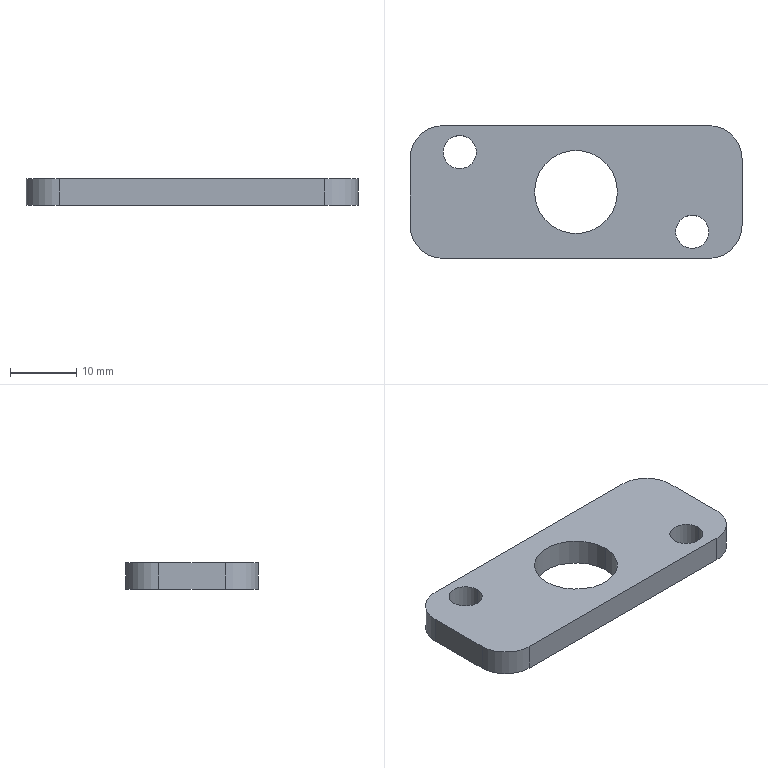Part | SolidWorks | features Extrusion 1 | 1 solid | 16 faces | box 50 x 20 x 4 mm | volume 3266 mm3 | cylinder 10 | plane 6 | commonest cylinder face diameters 5 x4 10 x4 12.5 x2
STEP:
#1=CARTESIAN_POINT('',(-6.25,0.,-2.));
#2=VERTEX_POINT('',#1);
#3=CARTESIAN_POINT('',(6.25,0.,-2.));
#4=VERTEX_POINT('',#3);
#5=CARTESIAN_POINT('',(0.,0.,-2.));
#6=DIRECTION('',(0.,0.,1.));
#7=DIRECTION('',(-1.,0.,0.));
#8=AXIS2_PLACEMENT_3D('',#5,#6,#7);
#9=CIRCLE('',#8,6.25);
#10=EDGE_CURVE('',#2,#4,#9,.T.);
#11=ORIENTED_EDGE('',*,*,#10,.F.);
#12=CARTESIAN_POINT('',(-6.25,0.,2.));
#13=VERTEX_POINT('',#12);
#14=CARTESIAN_POINT('',(-6.25,0.,-2.));
#15=DIRECTION('',(0.,0.,1.));
#16=VECTOR('',#15,1000.);
#17=LINE('',#14,#16);
#18=EDGE_CURVE('',#2,#13,#17,.T.);
#19=ORIENTED_EDGE('',*,*,#18,.T.);
#20=CARTESIAN_POINT('',(6.25,0.,2.));
#21=VERTEX_POINT('',#20);
#22=CARTESIAN_POINT('',(0.,0.,2.));
#23=DIRECTION('',(0.,0.,1.));
#24=DIRECTION('',(-1.,0.,0.));
#25=AXIS2_PLACEMENT_3D('',#22,#23,#24);
#26=CIRCLE('',#25,6.25);
#27=EDGE_CURVE('',#13,#21,#26,.T.);
#28=ORIENTED_EDGE('',*,*,#27,.T.);
#29=CARTESIAN_POINT('',(6.25,0.,-2.));
#30=DIRECTION('',(0.,0.,1.));
#31=VECTOR('',#30,1000.);
#32=LINE('',#29,#31);
#33=EDGE_CURVE('',#4,#21,#32,.T.);
#34=ORIENTED_EDGE('',*,*,#33,.F.);
#35=EDGE_LOOP('',(#11,#19,#28,#34));
#36=FACE_OUTER_BOUND('',#35,.T.);
#37=CARTESIAN_POINT('',(0.,0.,-2.));
#38=DIRECTION('',(0.,0.,1.));
#39=DIRECTION('',(1.,0.,0.));
#40=AXIS2_PLACEMENT_3D('',#37,#38,#39);
#41=CYLINDRICAL_SURFACE('',#40,6.25);
#42=ADVANCED_FACE('',(#36),#41,.F.);
#43=CARTESIAN_POINT('',(15.,-6.,-2.));
#44=VERTEX_POINT('',#43);
#45=CARTESIAN_POINT('',(20.,-6.,-2.));
#46=VERTEX_POINT('',#45);
#47=CARTESIAN_POINT('',(17.5,-6.,-2.));
#48=DIRECTION('',(0.,0.,1.));
#49=DIRECTION('',(-1.,0.,0.));
#50=AXIS2_PLACEMENT_3D('',#47,#48,#49);
#51=CIRCLE('',#50,2.5);
#52=EDGE_CURVE('',#44,#46,#51,.T.);
#53=ORIENTED_EDGE('',*,*,#52,.F.);
#54=CARTESIAN_POINT('',(15.,-6.,2.));
#55=VERTEX_POINT('',#54);
#56=CARTESIAN_POINT('',(15.,-6.,-2.));
#57=DIRECTION('',(0.,0.,1.));
#58=VECTOR('',#57,1000.);
#59=LINE('',#56,#58);
#60=EDGE_CURVE('',#44,#55,#59,.T.);
#61=ORIENTED_EDGE('',*,*,#60,.T.);
#62=CARTESIAN_POINT('',(20.,-6.,2.));
#63=VERTEX_POINT('',#62);
#64=CARTESIAN_POINT('',(17.5,-6.,2.));
#65=DIRECTION('',(0.,0.,1.));
#66=DIRECTION('',(-1.,0.,0.));
#67=AXIS2_PLACEMENT_3D('',#64,#65,#66);
#68=CIRCLE('',#67,2.5);
#69=EDGE_CURVE('',#55,#63,#68,.T.);
#70=ORIENTED_EDGE('',*,*,#69,.T.);
#71=CARTESIAN_POINT('',(20.,-6.,-2.));
#72=DIRECTION('',(0.,0.,1.));
#73=VECTOR('',#72,1000.);
#74=LINE('',#71,#73);
#75=EDGE_CURVE('',#46,#63,#74,.T.);
#76=ORIENTED_EDGE('',*,*,#75,.F.);
#77=EDGE_LOOP('',(#53,#61,#70,#76));
#78=FACE_OUTER_BOUND('',#77,.T.);
#79=CARTESIAN_POINT('',(17.5,-6.,-2.));
#80=DIRECTION('',(0.,0.,1.));
#81=DIRECTION('',(1.,0.,0.));
#82=AXIS2_PLACEMENT_3D('',#79,#80,#81);
#83=CYLINDRICAL_SURFACE('',#82,2.5);
#84=ADVANCED_FACE('',(#78),#83,.F.);
#85=CARTESIAN_POINT('',(-20.,6.,-2.));
#86=VERTEX_POINT('',#85);
#87=CARTESIAN_POINT('',(-15.,6.,-2.));
#88=VERTEX_POINT('',#87);
#89=CARTESIAN_POINT('',(-17.5,6.,-2.));
#90=DIRECTION('',(0.,0.,1.));
#91=DIRECTION('',(-1.,0.,0.));
#92=AXIS2_PLACEMENT_3D('',#89,#90,#91);
#93=CIRCLE('',#92,2.5);
#94=EDGE_CURVE('',#86,#88,#93,.T.);
#95=ORIENTED_EDGE('',*,*,#94,.F.);
#96=CARTESIAN_POINT('',(-20.,6.,2.));
#97=VERTEX_POINT('',#96);
#98=CARTESIAN_POINT('',(-20.,6.,-2.));
#99=DIRECTION('',(0.,0.,1.));
#100=VECTOR('',#99,1000.);
#101=LINE('',#98,#100);
#102=EDGE_CURVE('',#86,#97,#101,.T.);
#103=ORIENTED_EDGE('',*,*,#102,.T.);
#104=CARTESIAN_POINT('',(-15.,6.,2.));
#105=VERTEX_POINT('',#104);
#106=CARTESIAN_POINT('',(-17.5,6.,2.));
#107=DIRECTION('',(0.,0.,1.));
#108=DIRECTION('',(-1.,0.,0.));
#109=AXIS2_PLACEMENT_3D('',#106,#107,#108);
#110=CIRCLE('',#109,2.5);
#111=EDGE_CURVE('',#97,#105,#110,.T.);
#112=ORIENTED_EDGE('',*,*,#111,.T.);
#113=CARTESIAN_POINT('',(-15.,6.,-2.));
#114=DIRECTION('',(0.,0.,1.));
#115=VECTOR('',#114,1000.);
#116=LINE('',#113,#115);
#117=EDGE_CURVE('',#88,#105,#116,.T.);
#118=ORIENTED_EDGE('',*,*,#117,.F.);
#119=EDGE_LOOP('',(#95,#103,#112,#118));
#120=FACE_OUTER_BOUND('',#119,.T.);
#121=CARTESIAN_POINT('',(-17.5,6.,-2.));
#122=DIRECTION('',(0.,0.,1.));
#123=DIRECTION('',(1.,0.,0.));
#124=AXIS2_PLACEMENT_3D('',#121,#122,#123);
#125=CYLINDRICAL_SURFACE('',#124,2.5);
#126=ADVANCED_FACE('',(#120),#125,.F.);
#127=CARTESIAN_POINT('',(-25.,-5.,2.));
#128=VERTEX_POINT('',#127);
#129=CARTESIAN_POINT('',(-20.,-10.,2.));
#130=VERTEX_POINT('',#129);
#131=CARTESIAN_POINT('',(-20.,-5.,2.));
#132=DIRECTION('',(0.,0.,1.));
#133=DIRECTION('',(1.,0.,0.));
#134=AXIS2_PLACEMENT_3D('',#131,#132,#133);
#135=CIRCLE('',#134,5.);
#136=EDGE_CURVE('',#128,#130,#135,.T.);
#137=ORIENTED_EDGE('',*,*,#136,.F.);
#138=CARTESIAN_POINT('',(-25.,-5.,-2.));
#139=VERTEX_POINT('',#138);
#140=CARTESIAN_POINT('',(-25.,-5.,-2.));
#141=DIRECTION('',(0.,0.,1.));
#142=VECTOR('',#141,1000.);
#143=LINE('',#140,#142);
#144=EDGE_CURVE('',#139,#128,#143,.T.);
#145=ORIENTED_EDGE('',*,*,#144,.F.);
#146=CARTESIAN_POINT('',(-20.,-10.,-2.));
#147=VERTEX_POINT('',#146);
#148=CARTESIAN_POINT('',(-20.,-5.,-2.));
#149=DIRECTION('',(0.,0.,1.));
#150=DIRECTION('',(1.,0.,0.));
#151=AXIS2_PLACEMENT_3D('',#148,#149,#150);
#152=CIRCLE('',#151,5.);
#153=EDGE_CURVE('',#139,#147,#152,.T.);
#154=ORIENTED_EDGE('',*,*,#153,.T.);
#155=CARTESIAN_POINT('',(-20.,-10.,-2.));
#156=DIRECTION('',(0.,0.,1.));
#157=VECTOR('',#156,1000.);
#158=LINE('',#155,#157);
#159=EDGE_CURVE('',#147,#130,#158,.T.);
#160=ORIENTED_EDGE('',*,*,#159,.T.);
#161=EDGE_LOOP('',(#137,#145,#154,#160));
#162=FACE_OUTER_BOUND('',#161,.T.);
#163=CARTESIAN_POINT('',(-20.,-5.,-2.));
#164=DIRECTION('',(0.,0.,1.));
#165=DIRECTION('',(1.,0.,0.));
#166=AXIS2_PLACEMENT_3D('',#163,#164,#165);
#167=CYLINDRICAL_SURFACE('',#166,5.);
#168=ADVANCED_FACE('',(#162),#167,.T.);
#169=CARTESIAN_POINT('',(-25.,5.,2.));
#170=VERTEX_POINT('',#169);
#171=CARTESIAN_POINT('',(-25.,5.,2.));
#172=DIRECTION('',(0.,-1.,0.));
#173=VECTOR('',#172,1000.);
#174=LINE('',#171,#173);
#175=EDGE_CURVE('',#170,#128,#174,.T.);
#176=ORIENTED_EDGE('',*,*,#175,.F.);
#177=CARTESIAN_POINT('',(-25.,5.,-2.));
#178=VERTEX_POINT('',#177);
#179=CARTESIAN_POINT('',(-25.,5.,-2.));
#180=DIRECTION('',(0.,0.,1.));
#181=VECTOR('',#180,1000.);
#182=LINE('',#179,#181);
#183=EDGE_CURVE('',#178,#170,#182,.T.);
#184=ORIENTED_EDGE('',*,*,#183,.F.);
#185=CARTESIAN_POINT('',(-25.,5.,-2.));
#186=DIRECTION('',(0.,-1.,0.));
#187=VECTOR('',#186,1000.);
#188=LINE('',#185,#187);
#189=EDGE_CURVE('',#178,#139,#188,.T.);
#190=ORIENTED_EDGE('',*,*,#189,.T.);
#191=ORIENTED_EDGE('',*,*,#144,.T.);
#192=EDGE_LOOP('',(#176,#184,#190,#191));
#193=FACE_OUTER_BOUND('',#192,.T.);
#194=CARTESIAN_POINT('',(-25.,5.,-2.));
#195=DIRECTION('',(-1.,0.,0.));
#196=DIRECTION('',(0.,0.,1.));
#197=AXIS2_PLACEMENT_3D('',#194,#195,#196);
#198=PLANE('',#197);
#199=ADVANCED_FACE('',(#193),#198,.T.);
#200=CARTESIAN_POINT('',(-20.,10.,2.));
#201=VERTEX_POINT('',#200);
#202=CARTESIAN_POINT('',(-20.,5.,2.));
#203=DIRECTION('',(0.,0.,1.));
#204=DIRECTION('',(1.,0.,0.));
#205=AXIS2_PLACEMENT_3D('',#202,#203,#204);
#206=CIRCLE('',#205,5.);
#207=EDGE_CURVE('',#201,#170,#206,.T.);
#208=ORIENTED_EDGE('',*,*,#207,.F.);
#209=CARTESIAN_POINT('',(-20.,10.,-2.));
#210=VERTEX_POINT('',#209);
#211=CARTESIAN_POINT('',(-20.,10.,-2.));
#212=DIRECTION('',(0.,0.,1.));
#213=VECTOR('',#212,1000.);
#214=LINE('',#211,#213);
#215=EDGE_CURVE('',#210,#201,#214,.T.);
#216=ORIENTED_EDGE('',*,*,#215,.F.);
#217=CARTESIAN_POINT('',(-20.,5.,-2.));
#218=DIRECTION('',(0.,0.,1.));
#219=DIRECTION('',(1.,0.,0.));
#220=AXIS2_PLACEMENT_3D('',#217,#218,#219);
#221=CIRCLE('',#220,5.);
#222=EDGE_CURVE('',#210,#178,#221,.T.);
#223=ORIENTED_EDGE('',*,*,#222,.T.);
#224=ORIENTED_EDGE('',*,*,#183,.T.);
#225=EDGE_LOOP('',(#208,#216,#223,#224));
#226=FACE_OUTER_BOUND('',#225,.T.);
#227=CARTESIAN_POINT('',(-20.,5.,-2.));
#228=DIRECTION('',(0.,0.,1.));
#229=DIRECTION('',(1.,0.,0.));
#230=AXIS2_PLACEMENT_3D('',#227,#228,#229);
#231=CYLINDRICAL_SURFACE('',#230,5.);
#232=ADVANCED_FACE('',(#226),#231,.T.);
#233=CARTESIAN_POINT('',(20.,10.,2.));
#234=VERTEX_POINT('',#233);
#235=CARTESIAN_POINT('',(20.,10.,2.));
#236=DIRECTION('',(-1.,0.,0.));
#237=VECTOR('',#236,1000.);
#238=LINE('',#235,#237);
#239=EDGE_CURVE('',#234,#201,#238,.T.);
#240=ORIENTED_EDGE('',*,*,#239,.F.);
#241=CARTESIAN_POINT('',(20.,10.,-2.));
#242=VERTEX_POINT('',#241);
#243=CARTESIAN_POINT('',(20.,10.,-2.));
#244=DIRECTION('',(0.,0.,1.));
#245=VECTOR('',#244,1000.);
#246=LINE('',#243,#245);
#247=EDGE_CURVE('',#242,#234,#246,.T.);
#248=ORIENTED_EDGE('',*,*,#247,.F.);
#249=CARTESIAN_POINT('',(20.,10.,-2.));
#250=DIRECTION('',(-1.,0.,0.));
#251=VECTOR('',#250,1000.);
#252=LINE('',#249,#251);
#253=EDGE_CURVE('',#242,#210,#252,.T.);
#254=ORIENTED_EDGE('',*,*,#253,.T.);
#255=ORIENTED_EDGE('',*,*,#215,.T.);
#256=EDGE_LOOP('',(#240,#248,#254,#255));
#257=FACE_OUTER_BOUND('',#256,.T.);
#258=CARTESIAN_POINT('',(20.,10.,-2.));
#259=DIRECTION('',(0.,1.,0.));
#260=DIRECTION('',(0.,0.,1.));
#261=AXIS2_PLACEMENT_3D('',#258,#259,#260);
#262=PLANE('',#261);
#263=ADVANCED_FACE('',(#257),#262,.T.);
#264=CARTESIAN_POINT('',(25.,5.,2.));
#265=VERTEX_POINT('',#264);
#266=CARTESIAN_POINT('',(20.,5.,2.));
#267=DIRECTION('',(0.,0.,1.));
#268=DIRECTION('',(1.,0.,0.));
#269=AXIS2_PLACEMENT_3D('',#266,#267,#268);
#270=CIRCLE('',#269,5.);
#271=EDGE_CURVE('',#265,#234,#270,.T.);
#272=ORIENTED_EDGE('',*,*,#271,.F.);
#273=CARTESIAN_POINT('',(25.,5.,-2.));
#274=VERTEX_POINT('',#273);
#275=CARTESIAN_POINT('',(25.,5.,-2.));
#276=DIRECTION('',(0.,0.,1.));
#277=VECTOR('',#276,1000.);
#278=LINE('',#275,#277);
#279=EDGE_CURVE('',#274,#265,#278,.T.);
#280=ORIENTED_EDGE('',*,*,#279,.F.);
#281=CARTESIAN_POINT('',(20.,5.,-2.));
#282=DIRECTION('',(0.,0.,1.));
#283=DIRECTION('',(1.,0.,0.));
#284=AXIS2_PLACEMENT_3D('',#281,#282,#283);
#285=CIRCLE('',#284,5.);
#286=EDGE_CURVE('',#274,#242,#285,.T.);
#287=ORIENTED_EDGE('',*,*,#286,.T.);
#288=ORIENTED_EDGE('',*,*,#247,.T.);
#289=EDGE_LOOP('',(#272,#280,#287,#288));
#290=FACE_OUTER_BOUND('',#289,.T.);
#291=CARTESIAN_POINT('',(20.,5.,-2.));
#292=DIRECTION('',(0.,0.,1.));
#293=DIRECTION('',(1.,0.,0.));
#294=AXIS2_PLACEMENT_3D('',#291,#292,#293);
#295=CYLINDRICAL_SURFACE('',#294,5.);
#296=ADVANCED_FACE('',(#290),#295,.T.);
#297=CARTESIAN_POINT('',(25.,-5.,2.));
#298=VERTEX_POINT('',#297);
#299=CARTESIAN_POINT('',(25.,-5.,2.));
#300=DIRECTION('',(0.,1.,0.));
#301=VECTOR('',#300,1000.);
#302=LINE('',#299,#301);
#303=EDGE_CURVE('',#298,#265,#302,.T.);
#304=ORIENTED_EDGE('',*,*,#303,.F.);
#305=CARTESIAN_POINT('',(25.,-5.,-2.));
#306=VERTEX_POINT('',#305);
#307=CARTESIAN_POINT('',(25.,-5.,-2.));
#308=DIRECTION('',(0.,0.,1.));
#309=VECTOR('',#308,1000.);
#310=LINE('',#307,#309);
#311=EDGE_CURVE('',#306,#298,#310,.T.);
#312=ORIENTED_EDGE('',*,*,#311,.F.);
#313=CARTESIAN_POINT('',(25.,-5.,-2.));
#314=DIRECTION('',(0.,1.,0.));
#315=VECTOR('',#314,1000.);
#316=LINE('',#313,#315);
#317=EDGE_CURVE('',#306,#274,#316,.T.);
#318=ORIENTED_EDGE('',*,*,#317,.T.);
#319=ORIENTED_EDGE('',*,*,#279,.T.);
#320=EDGE_LOOP('',(#304,#312,#318,#319));
#321=FACE_OUTER_BOUND('',#320,.T.);
#322=CARTESIAN_POINT('',(25.,-5.,-2.));
#323=DIRECTION('',(1.,0.,0.));
#324=DIRECTION('',(0.,0.,-1.));
#325=AXIS2_PLACEMENT_3D('',#322,#323,#324);
#326=PLANE('',#325);
#327=ADVANCED_FACE('',(#321),#326,.T.);
#328=CARTESIAN_POINT('',(20.,-10.,2.));
#329=VERTEX_POINT('',#328);
#330=CARTESIAN_POINT('',(20.,-5.,2.));
#331=DIRECTION('',(0.,0.,1.));
#332=DIRECTION('',(1.,0.,0.));
#333=AXIS2_PLACEMENT_3D('',#330,#331,#332);
#334=CIRCLE('',#333,5.);
#335=EDGE_CURVE('',#329,#298,#334,.T.);
#336=ORIENTED_EDGE('',*,*,#335,.F.);
#337=CARTESIAN_POINT('',(20.,-10.,-2.));
#338=VERTEX_POINT('',#337);
#339=CARTESIAN_POINT('',(20.,-10.,-2.));
#340=DIRECTION('',(0.,0.,1.));
#341=VECTOR('',#340,1000.);
#342=LINE('',#339,#341);
#343=EDGE_CURVE('',#338,#329,#342,.T.);
#344=ORIENTED_EDGE('',*,*,#343,.F.);
#345=CARTESIAN_POINT('',(20.,-5.,-2.));
#346=DIRECTION('',(0.,0.,1.));
#347=DIRECTION('',(1.,0.,0.));
#348=AXIS2_PLACEMENT_3D('',#345,#346,#347);
#349=CIRCLE('',#348,5.);
#350=EDGE_CURVE('',#338,#306,#349,.T.);
#351=ORIENTED_EDGE('',*,*,#350,.T.);
#352=ORIENTED_EDGE('',*,*,#311,.T.);
#353=EDGE_LOOP('',(#336,#344,#351,#352));
#354=FACE_OUTER_BOUND('',#353,.T.);
#355=CARTESIAN_POINT('',(20.,-5.,-2.));
#356=DIRECTION('',(0.,0.,1.));
#357=DIRECTION('',(1.,0.,0.));
#358=AXIS2_PLACEMENT_3D('',#355,#356,#357);
#359=CYLINDRICAL_SURFACE('',#358,5.);
#360=ADVANCED_FACE('',(#354),#359,.T.);
#361=CARTESIAN_POINT('',(-20.,-10.,2.));
#362=DIRECTION('',(1.,0.,0.));
#363=VECTOR('',#362,1000.);
#364=LINE('',#361,#363);
#365=EDGE_CURVE('',#130,#329,#364,.T.);
#366=ORIENTED_EDGE('',*,*,#365,.F.);
#367=ORIENTED_EDGE('',*,*,#159,.F.);
#368=CARTESIAN_POINT('',(-20.,-10.,-2.));
#369=DIRECTION('',(1.,0.,0.));
#370=VECTOR('',#369,1000.);
#371=LINE('',#368,#370);
#372=EDGE_CURVE('',#147,#338,#371,.T.);
#373=ORIENTED_EDGE('',*,*,#372,.T.);
#374=ORIENTED_EDGE('',*,*,#343,.T.);
#375=EDGE_LOOP('',(#366,#367,#373,#374));
#376=FACE_OUTER_BOUND('',#375,.T.);
#377=CARTESIAN_POINT('',(-20.,-10.,-2.));
#378=DIRECTION('',(0.,-1.,0.));
#379=DIRECTION('',(0.,0.,-1.));
#380=AXIS2_PLACEMENT_3D('',#377,#378,#379);
#381=PLANE('',#380);
#382=ADVANCED_FACE('',(#376),#381,.T.);
#383=CARTESIAN_POINT('',(0.,0.,-2.));
#384=DIRECTION('',(0.,0.,1.));
#385=DIRECTION('',(-1.,0.,0.));
#386=AXIS2_PLACEMENT_3D('',#383,#384,#385);
#387=CIRCLE('',#386,6.25);
#388=EDGE_CURVE('',#4,#2,#387,.T.);
#389=ORIENTED_EDGE('',*,*,#388,.T.);
#390=ORIENTED_EDGE('',*,*,#10,.T.);
#391=EDGE_LOOP('',(#389,#390));
#392=FACE_BOUND('',#391,.T.);
#393=CARTESIAN_POINT('',(17.5,-6.,-2.));
#394=DIRECTION('',(0.,0.,1.));
#395=DIRECTION('',(-1.,0.,0.));
#396=AXIS2_PLACEMENT_3D('',#393,#394,#395);
#397=CIRCLE('',#396,2.5);
#398=EDGE_CURVE('',#46,#44,#397,.T.);
#399=ORIENTED_EDGE('',*,*,#398,.T.);
#400=ORIENTED_EDGE('',*,*,#52,.T.);
#401=EDGE_LOOP('',(#399,#400));
#402=FACE_BOUND('',#401,.T.);
#403=CARTESIAN_POINT('',(-17.5,6.,-2.));
#404=DIRECTION('',(0.,0.,1.));
#405=DIRECTION('',(-1.,0.,0.));
#406=AXIS2_PLACEMENT_3D('',#403,#404,#405);
#407=CIRCLE('',#406,2.5);
#408=EDGE_CURVE('',#88,#86,#407,.T.);
#409=ORIENTED_EDGE('',*,*,#408,.T.);
#410=ORIENTED_EDGE('',*,*,#94,.T.);
#411=EDGE_LOOP('',(#409,#410));
#412=FACE_BOUND('',#411,.T.);
#413=ORIENTED_EDGE('',*,*,#153,.F.);
#414=ORIENTED_EDGE('',*,*,#189,.F.);
#415=ORIENTED_EDGE('',*,*,#222,.F.);
#416=ORIENTED_EDGE('',*,*,#253,.F.);
#417=ORIENTED_EDGE('',*,*,#286,.F.);
#418=ORIENTED_EDGE('',*,*,#317,.F.);
#419=ORIENTED_EDGE('',*,*,#350,.F.);
#420=ORIENTED_EDGE('',*,*,#372,.F.);
#421=EDGE_LOOP('',(#413,#414,#415,#416,#417,#418,#419,#420));
#422=FACE_OUTER_BOUND('',#421,.T.);
#423=CARTESIAN_POINT('',(-20.,-5.,-2.));
#424=DIRECTION('',(0.,0.,1.));
#425=DIRECTION('',(1.,0.,0.));
#426=AXIS2_PLACEMENT_3D('',#423,#424,#425);
#427=PLANE('',#426);
#428=ADVANCED_FACE('',(#392,#402,#412,#422),#427,.F.);
#429=CARTESIAN_POINT('',(0.,0.,2.));
#430=DIRECTION('',(0.,0.,1.));
#431=DIRECTION('',(-1.,0.,0.));
#432=AXIS2_PLACEMENT_3D('',#429,#430,#431);
#433=CIRCLE('',#432,6.25);
#434=EDGE_CURVE('',#21,#13,#433,.T.);
#435=ORIENTED_EDGE('',*,*,#434,.F.);
#436=ORIENTED_EDGE('',*,*,#27,.F.);
#437=EDGE_LOOP('',(#435,#436));
#438=FACE_BOUND('',#437,.T.);
#439=CARTESIAN_POINT('',(17.5,-6.,2.));
#440=DIRECTION('',(0.,0.,1.));
#441=DIRECTION('',(-1.,0.,0.));
#442=AXIS2_PLACEMENT_3D('',#439,#440,#441);
#443=CIRCLE('',#442,2.5);
#444=EDGE_CURVE('',#63,#55,#443,.T.);
#445=ORIENTED_EDGE('',*,*,#444,.F.);
#446=ORIENTED_EDGE('',*,*,#69,.F.);
#447=EDGE_LOOP('',(#445,#446));
#448=FACE_BOUND('',#447,.T.);
#449=CARTESIAN_POINT('',(-17.5,6.,2.));
#450=DIRECTION('',(0.,0.,1.));
#451=DIRECTION('',(-1.,0.,0.));
#452=AXIS2_PLACEMENT_3D('',#449,#450,#451);
#453=CIRCLE('',#452,2.5);
#454=EDGE_CURVE('',#105,#97,#453,.T.);
#455=ORIENTED_EDGE('',*,*,#454,.F.);
#456=ORIENTED_EDGE('',*,*,#111,.F.);
#457=EDGE_LOOP('',(#455,#456));
#458=FACE_BOUND('',#457,.T.);
#459=ORIENTED_EDGE('',*,*,#136,.T.);
#460=ORIENTED_EDGE('',*,*,#365,.T.);
#461=ORIENTED_EDGE('',*,*,#335,.T.);
#462=ORIENTED_EDGE('',*,*,#303,.T.);
#463=ORIENTED_EDGE('',*,*,#271,.T.);
#464=ORIENTED_EDGE('',*,*,#239,.T.);
#465=ORIENTED_EDGE('',*,*,#207,.T.);
#466=ORIENTED_EDGE('',*,*,#175,.T.);
#467=EDGE_LOOP('',(#459,#460,#461,#462,#463,#464,#465,#466));
#468=FACE_OUTER_BOUND('',#467,.T.);
#469=CARTESIAN_POINT('',(-20.,-5.,2.));
#470=DIRECTION('',(0.,0.,1.));
#471=DIRECTION('',(1.,0.,0.));
#472=AXIS2_PLACEMENT_3D('',#469,#470,#471);
#473=PLANE('',#472);
#474=ADVANCED_FACE('',(#438,#448,#458,#468),#473,.T.);
#475=ORIENTED_EDGE('',*,*,#102,.F.);
#476=ORIENTED_EDGE('',*,*,#408,.F.);
#477=ORIENTED_EDGE('',*,*,#117,.T.);
#478=ORIENTED_EDGE('',*,*,#454,.T.);
#479=EDGE_LOOP('',(#475,#476,#477,#478));
#480=FACE_OUTER_BOUND('',#479,.T.);
#481=CARTESIAN_POINT('',(-17.5,6.,-2.));
#482=DIRECTION('',(0.,0.,1.));
#483=DIRECTION('',(1.,0.,0.));
#484=AXIS2_PLACEMENT_3D('',#481,#482,#483);
#485=CYLINDRICAL_SURFACE('',#484,2.5);
#486=ADVANCED_FACE('',(#480),#485,.F.);
#487=ORIENTED_EDGE('',*,*,#60,.F.);
#488=ORIENTED_EDGE('',*,*,#398,.F.);
#489=ORIENTED_EDGE('',*,*,#75,.T.);
#490=ORIENTED_EDGE('',*,*,#444,.T.);
#491=EDGE_LOOP('',(#487,#488,#489,#490));
#492=FACE_OUTER_BOUND('',#491,.T.);
#493=CARTESIAN_POINT('',(17.5,-6.,-2.));
#494=DIRECTION('',(0.,0.,1.));
#495=DIRECTION('',(1.,0.,0.));
#496=AXIS2_PLACEMENT_3D('',#493,#494,#495);
#497=CYLINDRICAL_SURFACE('',#496,2.5);
#498=ADVANCED_FACE('',(#492),#497,.F.);
#499=ORIENTED_EDGE('',*,*,#18,.F.);
#500=ORIENTED_EDGE('',*,*,#388,.F.);
#501=ORIENTED_EDGE('',*,*,#33,.T.);
#502=ORIENTED_EDGE('',*,*,#434,.T.);
#503=EDGE_LOOP('',(#499,#500,#501,#502));
#504=FACE_OUTER_BOUND('',#503,.T.);
#505=CARTESIAN_POINT('',(0.,0.,-2.));
#506=DIRECTION('',(0.,0.,1.));
#507=DIRECTION('',(1.,0.,0.));
#508=AXIS2_PLACEMENT_3D('',#505,#506,#507);
#509=CYLINDRICAL_SURFACE('',#508,6.25);
#510=ADVANCED_FACE('',(#504),#509,.F.);
#511=CLOSED_SHELL('',(#42,#84,#126,#168,#199,#232,#263,#296,#327,#360,#382,#428,#474,#486,#498,#510));
#512=MANIFOLD_SOLID_BREP('',#511);
#513=CARTESIAN_POINT('',(0.,0.,0.));
#514=DIRECTION('',(0.,0.,1.));
#515=DIRECTION('',(1.,0.,0.));
#516=AXIS2_PLACEMENT_3D('',#513,#514,#515);
#517=(LENGTH_UNIT()NAMED_UNIT(*)SI_UNIT(.MILLI.,.METRE.));
#518=UNCERTAINTY_MEASURE_WITH_UNIT(LENGTH_MEASURE(0.00001),#517,'','');
#519=(NAMED_UNIT(*)PLANE_ANGLE_UNIT()SI_UNIT($,.RADIAN.));
#520=(NAMED_UNIT(*)SI_UNIT($,.STERADIAN.)SOLID_ANGLE_UNIT());
#521=(GEOMETRIC_REPRESENTATION_CONTEXT(3)GLOBAL_UNCERTAINTY_ASSIGNED_CONTEXT((#518))GLOBAL_UNIT_ASSIGNED_CONTEXT((#517,#519,#520))REPRESENTATION_CONTEXT('',''));
#522=ADVANCED_BREP_SHAPE_REPRESENTATION('',(#512,#516),#521);